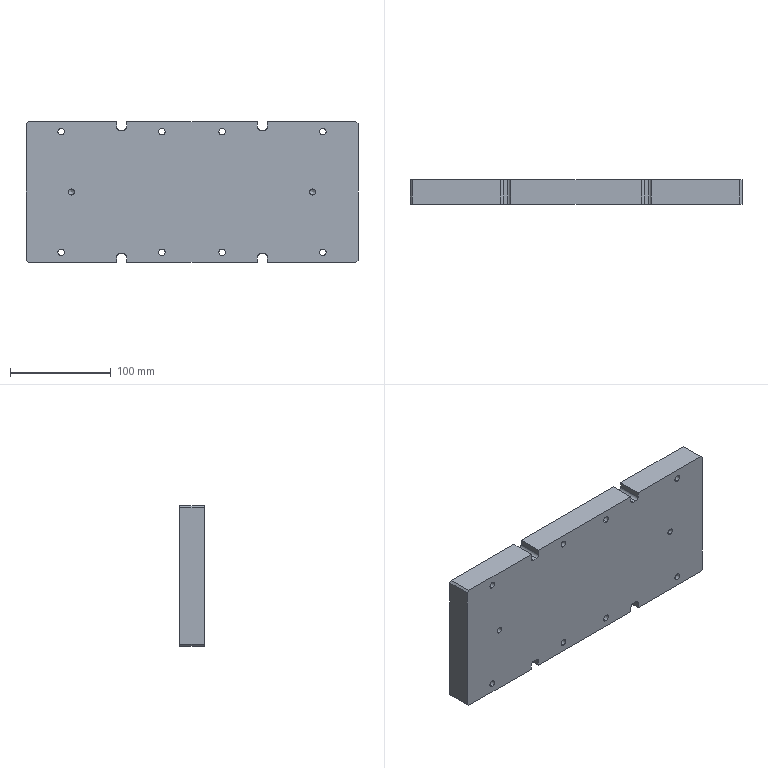Part | SolidWorks | features BaseBody 1 | 1 solid | 66 faces | box 330 x 24.5 x 140 mm | volume 1116300 mm3 | cylinder 32 | plane 26 | cone 8 | commonest cylinder face diameters 6 x16 6.6 x16